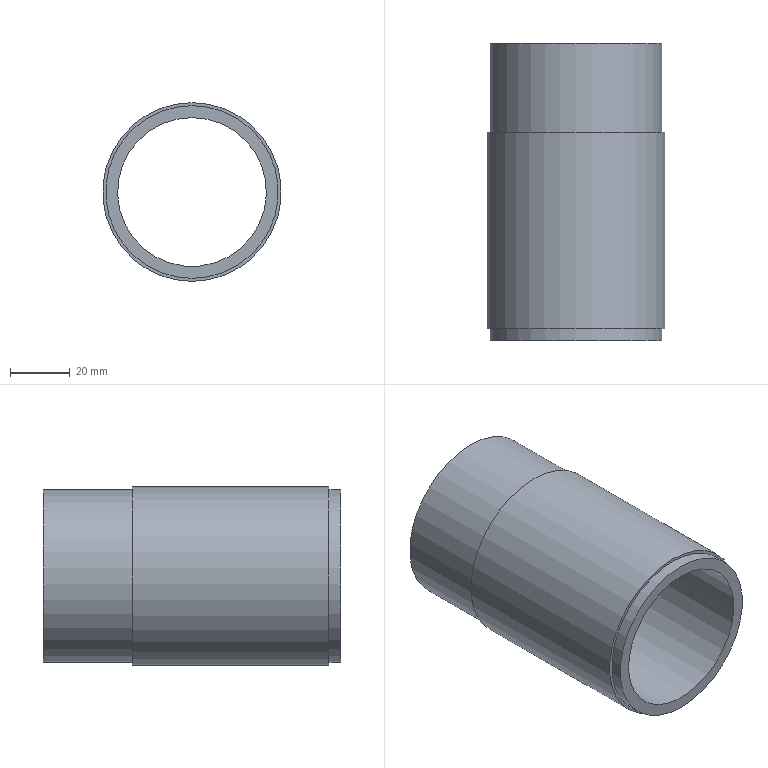Part | STEP file | JBJ-P-1009-01 | 1 solid | 8 faces | box 60 x 100 x 60 mm | volume 78768 mm3 | cylinder 4 | plane 3 | cone 1 | commonest cylinder face diameters 58 x2 50 x1 60 x1
STEP:
#1=CARTESIAN_POINT('',(0.,4.,-30.));
#2=VERTEX_POINT('',#1);
#3=CARTESIAN_POINT('',(0.,4.,0.));
#4=DIRECTION('',(0.,-1.,0.));
#5=DIRECTION('',(0.,0.,-1.));
#6=AXIS2_PLACEMENT_3D('',#3,#4,#5);
#7=CIRCLE('',#6,30.);
#8=EDGE_CURVE('',#2,#2,#7,.T.);
#9=ORIENTED_EDGE('',*,*,#8,.F.);
#10=EDGE_LOOP('',(#9));
#11=FACE_OUTER_BOUND('',#10,.T.);
#12=CARTESIAN_POINT('',(0.,70.,30.));
#13=VERTEX_POINT('',#12);
#14=CARTESIAN_POINT('',(0.,70.,0.));
#15=DIRECTION('',(0.,1.,0.));
#16=DIRECTION('',(0.,0.,1.));
#17=AXIS2_PLACEMENT_3D('',#14,#15,#16);
#18=CIRCLE('',#17,30.);
#19=EDGE_CURVE('',#13,#13,#18,.T.);
#20=ORIENTED_EDGE('',*,*,#19,.F.);
#21=EDGE_LOOP('',(#20));
#22=FACE_OUTER_BOUND('',#21,.T.);
#23=CARTESIAN_POINT('',(0.,100.,0.));
#24=DIRECTION('',(0.,-1.,0.));
#25=DIRECTION('',(0.,0.,-1.));
#26=AXIS2_PLACEMENT_3D('',#23,#24,#25);
#27=CYLINDRICAL_SURFACE('',#26,30.);
#28=ADVANCED_FACE('',(#11,#22),#27,.T.);
#29=CARTESIAN_POINT('',(0.,0.,25.));
#30=VERTEX_POINT('',#29);
#31=CARTESIAN_POINT('',(0.,0.,0.));
#32=DIRECTION('',(0.,1.,0.));
#33=DIRECTION('',(0.,0.,1.));
#34=AXIS2_PLACEMENT_3D('',#31,#32,#33);
#35=CIRCLE('',#34,25.);
#36=EDGE_CURVE('',#30,#30,#35,.T.);
#37=ORIENTED_EDGE('',*,*,#36,.T.);
#38=EDGE_LOOP('',(#37));
#39=FACE_BOUND('',#38,.T.);
#40=CARTESIAN_POINT('',(0.,0.,-29.));
#41=VERTEX_POINT('',#40);
#42=CARTESIAN_POINT('',(0.,0.,0.));
#43=DIRECTION('',(0.,-1.,0.));
#44=DIRECTION('',(0.,0.,-1.));
#45=AXIS2_PLACEMENT_3D('',#42,#43,#44);
#46=CIRCLE('',#45,29.);
#47=EDGE_CURVE('',#41,#41,#46,.T.);
#48=ORIENTED_EDGE('',*,*,#47,.T.);
#49=EDGE_LOOP('',(#48));
#50=FACE_OUTER_BOUND('',#49,.T.);
#51=CARTESIAN_POINT('',(0.,0.,0.));
#52=DIRECTION('',(0.,1.,0.));
#53=DIRECTION('',(0.,0.,1.));
#54=AXIS2_PLACEMENT_3D('',#51,#52,#53);
#55=PLANE('',#54);
#56=ADVANCED_FACE('',(#39,#50),#55,.F.);
#57=CARTESIAN_POINT('',(0.,96.,25.));
#58=VERTEX_POINT('',#57);
#59=CARTESIAN_POINT('',(0.,96.,0.));
#60=DIRECTION('',(0.,1.,0.));
#61=DIRECTION('',(0.,0.,1.));
#62=AXIS2_PLACEMENT_3D('',#59,#60,#61);
#63=CIRCLE('',#62,25.);
#64=EDGE_CURVE('',#58,#58,#63,.T.);
#65=ORIENTED_EDGE('',*,*,#64,.T.);
#66=EDGE_LOOP('',(#65));
#67=FACE_OUTER_BOUND('',#66,.T.);
#68=ORIENTED_EDGE('',*,*,#36,.F.);
#69=EDGE_LOOP('',(#68));
#70=FACE_OUTER_BOUND('',#69,.T.);
#71=CARTESIAN_POINT('',(0.,100.,0.));
#72=DIRECTION('',(0.,-1.,0.));
#73=DIRECTION('',(0.,0.,-1.));
#74=AXIS2_PLACEMENT_3D('',#71,#72,#73);
#75=CYLINDRICAL_SURFACE('',#74,25.);
#76=ADVANCED_FACE('',(#67,#70),#75,.F.);
#77=CARTESIAN_POINT('',(0.,4.,-29.));
#78=VERTEX_POINT('',#77);
#79=CARTESIAN_POINT('',(0.,4.,0.));
#80=DIRECTION('',(0.,-1.,0.));
#81=DIRECTION('',(0.,0.,-1.));
#82=AXIS2_PLACEMENT_3D('',#79,#80,#81);
#83=CIRCLE('',#82,29.);
#84=EDGE_CURVE('',#78,#78,#83,.T.);
#85=ORIENTED_EDGE('',*,*,#84,.F.);
#86=EDGE_LOOP('',(#85));
#87=FACE_BOUND('',#86,.T.);
#88=ORIENTED_EDGE('',*,*,#8,.T.);
#89=EDGE_LOOP('',(#88));
#90=FACE_OUTER_BOUND('',#89,.T.);
#91=CARTESIAN_POINT('',(0.,4.,0.));
#92=DIRECTION('',(0.,-1.,0.));
#93=DIRECTION('',(0.,0.,-1.));
#94=AXIS2_PLACEMENT_3D('',#91,#92,#93);
#95=PLANE('',#94);
#96=ADVANCED_FACE('',(#87,#90),#95,.T.);
#97=ORIENTED_EDGE('',*,*,#84,.T.);
#98=EDGE_LOOP('',(#97));
#99=FACE_OUTER_BOUND('',#98,.T.);
#100=ORIENTED_EDGE('',*,*,#47,.F.);
#101=EDGE_LOOP('',(#100));
#102=FACE_OUTER_BOUND('',#101,.T.);
#103=CARTESIAN_POINT('',(0.,4.,0.));
#104=DIRECTION('',(0.,-1.,0.));
#105=DIRECTION('',(0.,0.,-1.));
#106=AXIS2_PLACEMENT_3D('',#103,#104,#105);
#107=CYLINDRICAL_SURFACE('',#106,29.);
#108=ADVANCED_FACE('',(#99,#102),#107,.T.);
#109=CARTESIAN_POINT('',(0.,70.,29.));
#110=VERTEX_POINT('',#109);
#111=CARTESIAN_POINT('',(0.,70.,0.));
#112=DIRECTION('',(0.,1.,0.));
#113=DIRECTION('',(0.,0.,1.));
#114=AXIS2_PLACEMENT_3D('',#111,#112,#113);
#115=CIRCLE('',#114,29.);
#116=EDGE_CURVE('',#110,#110,#115,.T.);
#117=ORIENTED_EDGE('',*,*,#116,.F.);
#118=EDGE_LOOP('',(#117));
#119=FACE_BOUND('',#118,.T.);
#120=ORIENTED_EDGE('',*,*,#19,.T.);
#121=EDGE_LOOP('',(#120));
#122=FACE_OUTER_BOUND('',#121,.T.);
#123=CARTESIAN_POINT('',(0.,70.,0.));
#124=DIRECTION('',(0.,1.,0.));
#125=DIRECTION('',(0.,0.,1.));
#126=AXIS2_PLACEMENT_3D('',#123,#124,#125);
#127=PLANE('',#126);
#128=ADVANCED_FACE('',(#119,#122),#127,.T.);
#129=ORIENTED_EDGE('',*,*,#116,.T.);
#130=EDGE_LOOP('',(#129));
#131=FACE_OUTER_BOUND('',#130,.T.);
#132=CARTESIAN_POINT('',(0.,100.,29.));
#133=VERTEX_POINT('',#132);
#134=CARTESIAN_POINT('',(0.,100.,0.));
#135=DIRECTION('',(0.,1.,0.));
#136=DIRECTION('',(0.,0.,1.));
#137=AXIS2_PLACEMENT_3D('',#134,#135,#136);
#138=CIRCLE('',#137,29.);
#139=EDGE_CURVE('',#133,#133,#138,.T.);
#140=ORIENTED_EDGE('',*,*,#139,.F.);
#141=EDGE_LOOP('',(#140));
#142=FACE_OUTER_BOUND('',#141,.T.);
#143=CARTESIAN_POINT('',(0.,70.,0.));
#144=DIRECTION('',(0.,1.,0.));
#145=DIRECTION('',(0.,0.,1.));
#146=AXIS2_PLACEMENT_3D('',#143,#144,#145);
#147=CYLINDRICAL_SURFACE('',#146,29.);
#148=ADVANCED_FACE('',(#131,#142),#147,.T.);
#149=ORIENTED_EDGE('',*,*,#139,.T.);
#150=EDGE_LOOP('',(#149));
#151=FACE_OUTER_BOUND('',#150,.T.);
#152=ORIENTED_EDGE('',*,*,#64,.F.);
#153=EDGE_LOOP('',(#152));
#154=FACE_BOUND('',#153,.T.);
#155=CARTESIAN_POINT('',(0.,96.,0.));
#156=DIRECTION('',(0.,1.,0.));
#157=DIRECTION('',(0.,0.,1.));
#158=AXIS2_PLACEMENT_3D('',#155,#156,#157);
#159=CONICAL_SURFACE('',#158,25.,0.7854);
#160=ADVANCED_FACE('',(#151,#154),#159,.F.);
#161=CLOSED_SHELL('',(#28,#56,#76,#96,#108,#128,#148,#160));
#162=MANIFOLD_SOLID_BREP('',#161);
#163=CARTESIAN_POINT('',(0.,0.,0.));
#164=DIRECTION('',(0.,0.,1.));
#165=DIRECTION('',(1.,0.,0.));
#166=AXIS2_PLACEMENT_3D('',#163,#164,#165);
#167=(LENGTH_UNIT()NAMED_UNIT(*)SI_UNIT(.MILLI.,.METRE.));
#168=UNCERTAINTY_MEASURE_WITH_UNIT(LENGTH_MEASURE(0.00001),#167,'','');
#169=(NAMED_UNIT(*)PLANE_ANGLE_UNIT()SI_UNIT($,.RADIAN.));
#170=(NAMED_UNIT(*)SI_UNIT($,.STERADIAN.)SOLID_ANGLE_UNIT());
#171=(GEOMETRIC_REPRESENTATION_CONTEXT(3)GLOBAL_UNCERTAINTY_ASSIGNED_CONTEXT((#168))GLOBAL_UNIT_ASSIGNED_CONTEXT((#167,#169,#170))REPRESENTATION_CONTEXT('',''));
#172=ADVANCED_BREP_SHAPE_REPRESENTATION('',(#162,#166),#171);